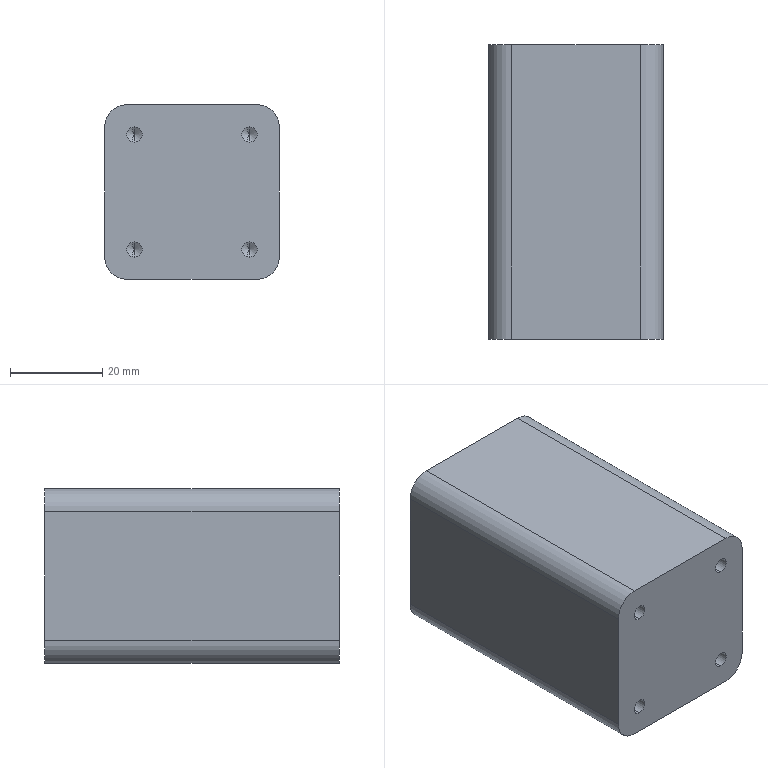Part | SolidWorks | features HoleWzd 2, ICE 2, Extrusion 1, Fillet 1 | 1 solid | 42 faces | box 38 x 64 x 38 mm | volume 90329 mm3 | cylinder 20 | cone 16 | plane 6 | commonest cylinder face diameters 3.3 x16 10 x4
STEP:
#1=CARTESIAN_POINT('',(-12.5,53.9,-14.15));
#2=VERTEX_POINT('',#1);
#3=CARTESIAN_POINT('',(-12.5,53.9,-10.85));
#4=VERTEX_POINT('',#3);
#5=CARTESIAN_POINT('',(-12.5,53.9,-12.5));
#6=DIRECTION('',(0.,1.,0.));
#7=DIRECTION('',(0.,0.,1.));
#8=AXIS2_PLACEMENT_3D('',#5,#6,#7);
#9=CIRCLE('',#8,1.65);
#10=EDGE_CURVE('',#2,#4,#9,.T.);
#11=ORIENTED_EDGE('',*,*,#10,.F.);
#12=CARTESIAN_POINT('',(-12.5,64.,-14.15));
#13=VERTEX_POINT('',#12);
#14=CARTESIAN_POINT('',(-12.5,64.,-14.15));
#15=DIRECTION('',(0.,1.,0.));
#16=VECTOR('',#15,1000.);
#17=LINE('',#14,#16);
#18=EDGE_CURVE('',#2,#13,#17,.T.);
#19=ORIENTED_EDGE('',*,*,#18,.T.);
#20=CARTESIAN_POINT('',(-12.5,64.,-10.85));
#21=VERTEX_POINT('',#20);
#22=CARTESIAN_POINT('',(-12.5,64.,-12.5));
#23=DIRECTION('',(0.,1.,0.));
#24=DIRECTION('',(0.,0.,1.));
#25=AXIS2_PLACEMENT_3D('',#22,#23,#24);
#26=CIRCLE('',#25,1.65);
#27=EDGE_CURVE('',#13,#21,#26,.T.);
#28=ORIENTED_EDGE('',*,*,#27,.T.);
#29=CARTESIAN_POINT('',(-12.5,64.,-10.85));
#30=DIRECTION('',(0.,1.,0.));
#31=VECTOR('',#30,1000.);
#32=LINE('',#29,#31);
#33=EDGE_CURVE('',#4,#21,#32,.T.);
#34=ORIENTED_EDGE('',*,*,#33,.F.);
#35=EDGE_LOOP('',(#11,#19,#28,#34));
#36=FACE_OUTER_BOUND('',#35,.T.);
#37=CARTESIAN_POINT('',(-12.5,64.,-12.5));
#38=DIRECTION('',(0.,1.,0.));
#39=DIRECTION('',(0.,0.,1.));
#40=AXIS2_PLACEMENT_3D('',#37,#38,#39);
#41=CYLINDRICAL_SURFACE('',#40,1.65);
#42=ADVANCED_FACE('',(#36),#41,.F.);
#43=CARTESIAN_POINT('',(-12.5,52.909,-12.5));
#44=VERTEX_POINT('',#43);
#45=CARTESIAN_POINT('',(-12.5,53.9,-10.85));
#46=DIRECTION('',(0.,0.515,0.8572));
#47=VECTOR('',#46,1000.);
#48=LINE('',#45,#47);
#49=EDGE_CURVE('',#44,#4,#48,.T.);
#50=ORIENTED_EDGE('',*,*,#49,.F.);
#51=CARTESIAN_POINT('',(-12.5,53.9,-14.15));
#52=DIRECTION('',(0.,0.515,-0.8572));
#53=VECTOR('',#52,1000.);
#54=LINE('',#51,#53);
#55=EDGE_CURVE('',#44,#2,#54,.T.);
#56=ORIENTED_EDGE('',*,*,#55,.T.);
#57=ORIENTED_EDGE('',*,*,#10,.T.);
#58=EDGE_LOOP('',(#50,#56,#57));
#59=FACE_OUTER_BOUND('',#58,.T.);
#60=CARTESIAN_POINT('',(-12.5,53.9,-12.5));
#61=DIRECTION('',(0.,1.,0.));
#62=DIRECTION('',(0.,0.,1.));
#63=AXIS2_PLACEMENT_3D('',#60,#61,#62);
#64=CONICAL_SURFACE('',#63,1.65,1.03);
#65=ADVANCED_FACE('',(#59),#64,.F.);
#66=CARTESIAN_POINT('',(12.5,53.9,-14.15));
#67=VERTEX_POINT('',#66);
#68=CARTESIAN_POINT('',(12.5,53.9,-10.85));
#69=VERTEX_POINT('',#68);
#70=CARTESIAN_POINT('',(12.5,53.9,-12.5));
#71=DIRECTION('',(0.,1.,0.));
#72=DIRECTION('',(0.,0.,1.));
#73=AXIS2_PLACEMENT_3D('',#70,#71,#72);
#74=CIRCLE('',#73,1.65);
#75=EDGE_CURVE('',#67,#69,#74,.T.);
#76=ORIENTED_EDGE('',*,*,#75,.F.);
#77=CARTESIAN_POINT('',(12.5,64.,-14.15));
#78=VERTEX_POINT('',#77);
#79=CARTESIAN_POINT('',(12.5,64.,-14.15));
#80=DIRECTION('',(0.,1.,0.));
#81=VECTOR('',#80,1000.);
#82=LINE('',#79,#81);
#83=EDGE_CURVE('',#67,#78,#82,.T.);
#84=ORIENTED_EDGE('',*,*,#83,.T.);
#85=CARTESIAN_POINT('',(12.5,64.,-10.85));
#86=VERTEX_POINT('',#85);
#87=CARTESIAN_POINT('',(12.5,64.,-12.5));
#88=DIRECTION('',(0.,1.,0.));
#89=DIRECTION('',(0.,0.,1.));
#90=AXIS2_PLACEMENT_3D('',#87,#88,#89);
#91=CIRCLE('',#90,1.65);
#92=EDGE_CURVE('',#78,#86,#91,.T.);
#93=ORIENTED_EDGE('',*,*,#92,.T.);
#94=CARTESIAN_POINT('',(12.5,64.,-10.85));
#95=DIRECTION('',(0.,1.,0.));
#96=VECTOR('',#95,1000.);
#97=LINE('',#94,#96);
#98=EDGE_CURVE('',#69,#86,#97,.T.);
#99=ORIENTED_EDGE('',*,*,#98,.F.);
#100=EDGE_LOOP('',(#76,#84,#93,#99));
#101=FACE_OUTER_BOUND('',#100,.T.);
#102=CARTESIAN_POINT('',(12.5,64.,-12.5));
#103=DIRECTION('',(0.,1.,0.));
#104=DIRECTION('',(0.,0.,1.));
#105=AXIS2_PLACEMENT_3D('',#102,#103,#104);
#106=CYLINDRICAL_SURFACE('',#105,1.65);
#107=ADVANCED_FACE('',(#101),#106,.F.);
#108=CARTESIAN_POINT('',(12.5,52.909,-12.5));
#109=VERTEX_POINT('',#108);
#110=CARTESIAN_POINT('',(12.5,53.9,-10.85));
#111=DIRECTION('',(0.,0.515,0.8572));
#112=VECTOR('',#111,1000.);
#113=LINE('',#110,#112);
#114=EDGE_CURVE('',#109,#69,#113,.T.);
#115=ORIENTED_EDGE('',*,*,#114,.F.);
#116=CARTESIAN_POINT('',(12.5,53.9,-14.15));
#117=DIRECTION('',(0.,0.515,-0.8572));
#118=VECTOR('',#117,1000.);
#119=LINE('',#116,#118);
#120=EDGE_CURVE('',#109,#67,#119,.T.);
#121=ORIENTED_EDGE('',*,*,#120,.T.);
#122=ORIENTED_EDGE('',*,*,#75,.T.);
#123=EDGE_LOOP('',(#115,#121,#122));
#124=FACE_OUTER_BOUND('',#123,.T.);
#125=CARTESIAN_POINT('',(12.5,53.9,-12.5));
#126=DIRECTION('',(0.,1.,0.));
#127=DIRECTION('',(0.,0.,1.));
#128=AXIS2_PLACEMENT_3D('',#125,#126,#127);
#129=CONICAL_SURFACE('',#128,1.65,1.03);
#130=ADVANCED_FACE('',(#124),#129,.F.);
#131=CARTESIAN_POINT('',(12.5,53.9,10.85));
#132=VERTEX_POINT('',#131);
#133=CARTESIAN_POINT('',(12.5,53.9,14.15));
#134=VERTEX_POINT('',#133);
#135=CARTESIAN_POINT('',(12.5,53.9,12.5));
#136=DIRECTION('',(0.,1.,0.));
#137=DIRECTION('',(0.,0.,1.));
#138=AXIS2_PLACEMENT_3D('',#135,#136,#137);
#139=CIRCLE('',#138,1.65);
#140=EDGE_CURVE('',#132,#134,#139,.T.);
#141=ORIENTED_EDGE('',*,*,#140,.F.);
#142=CARTESIAN_POINT('',(12.5,64.,10.85));
#143=VERTEX_POINT('',#142);
#144=CARTESIAN_POINT('',(12.5,64.,10.85));
#145=DIRECTION('',(0.,1.,0.));
#146=VECTOR('',#145,1000.);
#147=LINE('',#144,#146);
#148=EDGE_CURVE('',#132,#143,#147,.T.);
#149=ORIENTED_EDGE('',*,*,#148,.T.);
#150=CARTESIAN_POINT('',(12.5,64.,14.15));
#151=VERTEX_POINT('',#150);
#152=CARTESIAN_POINT('',(12.5,64.,12.5));
#153=DIRECTION('',(0.,1.,0.));
#154=DIRECTION('',(0.,0.,1.));
#155=AXIS2_PLACEMENT_3D('',#152,#153,#154);
#156=CIRCLE('',#155,1.65);
#157=EDGE_CURVE('',#143,#151,#156,.T.);
#158=ORIENTED_EDGE('',*,*,#157,.T.);
#159=CARTESIAN_POINT('',(12.5,64.,14.15));
#160=DIRECTION('',(0.,1.,0.));
#161=VECTOR('',#160,1000.);
#162=LINE('',#159,#161);
#163=EDGE_CURVE('',#134,#151,#162,.T.);
#164=ORIENTED_EDGE('',*,*,#163,.F.);
#165=EDGE_LOOP('',(#141,#149,#158,#164));
#166=FACE_OUTER_BOUND('',#165,.T.);
#167=CARTESIAN_POINT('',(12.5,64.,12.5));
#168=DIRECTION('',(0.,1.,0.));
#169=DIRECTION('',(0.,0.,1.));
#170=AXIS2_PLACEMENT_3D('',#167,#168,#169);
#171=CYLINDRICAL_SURFACE('',#170,1.65);
#172=ADVANCED_FACE('',(#166),#171,.F.);
#173=CARTESIAN_POINT('',(12.5,52.909,12.5));
#174=VERTEX_POINT('',#173);
#175=CARTESIAN_POINT('',(12.5,53.9,14.15));
#176=DIRECTION('',(0.,0.515,0.8572));
#177=VECTOR('',#176,1000.);
#178=LINE('',#175,#177);
#179=EDGE_CURVE('',#174,#134,#178,.T.);
#180=ORIENTED_EDGE('',*,*,#179,.F.);
#181=CARTESIAN_POINT('',(12.5,53.9,10.85));
#182=DIRECTION('',(0.,0.515,-0.8572));
#183=VECTOR('',#182,1000.);
#184=LINE('',#181,#183);
#185=EDGE_CURVE('',#174,#132,#184,.T.);
#186=ORIENTED_EDGE('',*,*,#185,.T.);
#187=ORIENTED_EDGE('',*,*,#140,.T.);
#188=EDGE_LOOP('',(#180,#186,#187));
#189=FACE_OUTER_BOUND('',#188,.T.);
#190=CARTESIAN_POINT('',(12.5,53.9,12.5));
#191=DIRECTION('',(0.,1.,0.));
#192=DIRECTION('',(0.,0.,1.));
#193=AXIS2_PLACEMENT_3D('',#190,#191,#192);
#194=CONICAL_SURFACE('',#193,1.65,1.03);
#195=ADVANCED_FACE('',(#189),#194,.F.);
#196=CARTESIAN_POINT('',(-12.5,53.9,10.85));
#197=VERTEX_POINT('',#196);
#198=CARTESIAN_POINT('',(-12.5,53.9,14.15));
#199=VERTEX_POINT('',#198);
#200=CARTESIAN_POINT('',(-12.5,53.9,12.5));
#201=DIRECTION('',(0.,1.,0.));
#202=DIRECTION('',(0.,0.,1.));
#203=AXIS2_PLACEMENT_3D('',#200,#201,#202);
#204=CIRCLE('',#203,1.65);
#205=EDGE_CURVE('',#197,#199,#204,.T.);
#206=ORIENTED_EDGE('',*,*,#205,.F.);
#207=CARTESIAN_POINT('',(-12.5,64.,10.85));
#208=VERTEX_POINT('',#207);
#209=CARTESIAN_POINT('',(-12.5,64.,10.85));
#210=DIRECTION('',(0.,1.,0.));
#211=VECTOR('',#210,1000.);
#212=LINE('',#209,#211);
#213=EDGE_CURVE('',#197,#208,#212,.T.);
#214=ORIENTED_EDGE('',*,*,#213,.T.);
#215=CARTESIAN_POINT('',(-12.5,64.,14.15));
#216=VERTEX_POINT('',#215);
#217=CARTESIAN_POINT('',(-12.5,64.,12.5));
#218=DIRECTION('',(0.,1.,0.));
#219=DIRECTION('',(0.,0.,1.));
#220=AXIS2_PLACEMENT_3D('',#217,#218,#219);
#221=CIRCLE('',#220,1.65);
#222=EDGE_CURVE('',#208,#216,#221,.T.);
#223=ORIENTED_EDGE('',*,*,#222,.T.);
#224=CARTESIAN_POINT('',(-12.5,64.,14.15));
#225=DIRECTION('',(0.,1.,0.));
#226=VECTOR('',#225,1000.);
#227=LINE('',#224,#226);
#228=EDGE_CURVE('',#199,#216,#227,.T.);
#229=ORIENTED_EDGE('',*,*,#228,.F.);
#230=EDGE_LOOP('',(#206,#214,#223,#229));
#231=FACE_OUTER_BOUND('',#230,.T.);
#232=CARTESIAN_POINT('',(-12.5,64.,12.5));
#233=DIRECTION('',(0.,1.,0.));
#234=DIRECTION('',(0.,0.,1.));
#235=AXIS2_PLACEMENT_3D('',#232,#233,#234);
#236=CYLINDRICAL_SURFACE('',#235,1.65);
#237=ADVANCED_FACE('',(#231),#236,.F.);
#238=CARTESIAN_POINT('',(-12.5,52.909,12.5));
#239=VERTEX_POINT('',#238);
#240=CARTESIAN_POINT('',(-12.5,53.9,14.15));
#241=DIRECTION('',(0.,0.515,0.8572));
#242=VECTOR('',#241,1000.);
#243=LINE('',#240,#242);
#244=EDGE_CURVE('',#239,#199,#243,.T.);
#245=ORIENTED_EDGE('',*,*,#244,.F.);
#246=CARTESIAN_POINT('',(-12.5,53.9,10.85));
#247=DIRECTION('',(0.,0.515,-0.8572));
#248=VECTOR('',#247,1000.);
#249=LINE('',#246,#248);
#250=EDGE_CURVE('',#239,#197,#249,.T.);
#251=ORIENTED_EDGE('',*,*,#250,.T.);
#252=ORIENTED_EDGE('',*,*,#205,.T.);
#253=EDGE_LOOP('',(#245,#251,#252));
#254=FACE_OUTER_BOUND('',#253,.T.);
#255=CARTESIAN_POINT('',(-12.5,53.9,12.5));
#256=DIRECTION('',(0.,1.,0.));
#257=DIRECTION('',(0.,0.,1.));
#258=AXIS2_PLACEMENT_3D('',#255,#256,#257);
#259=CONICAL_SURFACE('',#258,1.65,1.03);
#260=ADVANCED_FACE('',(#254),#259,.F.);
#261=CARTESIAN_POINT('',(-12.5,10.1,-10.85));
#262=VERTEX_POINT('',#261);
#263=CARTESIAN_POINT('',(-12.5,10.1,-14.15));
#264=VERTEX_POINT('',#263);
#265=CARTESIAN_POINT('',(-12.5,10.1,-12.5));
#266=DIRECTION('',(0.,-1.,0.));
#267=DIRECTION('',(0.,0.,-1.));
#268=AXIS2_PLACEMENT_3D('',#265,#266,#267);
#269=CIRCLE('',#268,1.65);
#270=EDGE_CURVE('',#262,#264,#269,.T.);
#271=ORIENTED_EDGE('',*,*,#270,.F.);
#272=CARTESIAN_POINT('',(-12.5,0.,-10.85));
#273=VERTEX_POINT('',#272);
#274=CARTESIAN_POINT('',(-12.5,0.,-10.85));
#275=DIRECTION('',(0.,-1.,0.));
#276=VECTOR('',#275,1000.);
#277=LINE('',#274,#276);
#278=EDGE_CURVE('',#262,#273,#277,.T.);
#279=ORIENTED_EDGE('',*,*,#278,.T.);
#280=CARTESIAN_POINT('',(-12.5,0.,-14.15));
#281=VERTEX_POINT('',#280);
#282=CARTESIAN_POINT('',(-12.5,0.,-12.5));
#283=DIRECTION('',(0.,-1.,0.));
#284=DIRECTION('',(0.,0.,-1.));
#285=AXIS2_PLACEMENT_3D('',#282,#283,#284);
#286=CIRCLE('',#285,1.65);
#287=EDGE_CURVE('',#273,#281,#286,.T.);
#288=ORIENTED_EDGE('',*,*,#287,.T.);
#289=CARTESIAN_POINT('',(-12.5,0.,-14.15));
#290=DIRECTION('',(0.,-1.,0.));
#291=VECTOR('',#290,1000.);
#292=LINE('',#289,#291);
#293=EDGE_CURVE('',#264,#281,#292,.T.);
#294=ORIENTED_EDGE('',*,*,#293,.F.);
#295=EDGE_LOOP('',(#271,#279,#288,#294));
#296=FACE_OUTER_BOUND('',#295,.T.);
#297=CARTESIAN_POINT('',(-12.5,0.,-12.5));
#298=DIRECTION('',(0.,-1.,0.));
#299=DIRECTION('',(0.,0.,-1.));
#300=AXIS2_PLACEMENT_3D('',#297,#298,#299);
#301=CYLINDRICAL_SURFACE('',#300,1.65);
#302=ADVANCED_FACE('',(#296),#301,.F.);
#303=CARTESIAN_POINT('',(-12.5,11.091,-12.5));
#304=VERTEX_POINT('',#303);
#305=CARTESIAN_POINT('',(-12.5,10.1,-14.15));
#306=DIRECTION('',(0.,-0.515,-0.8572));
#307=VECTOR('',#306,1000.);
#308=LINE('',#305,#307);
#309=EDGE_CURVE('',#304,#264,#308,.T.);
#310=ORIENTED_EDGE('',*,*,#309,.F.);
#311=CARTESIAN_POINT('',(-12.5,10.1,-10.85));
#312=DIRECTION('',(0.,-0.515,0.8572));
#313=VECTOR('',#312,1000.);
#314=LINE('',#311,#313);
#315=EDGE_CURVE('',#304,#262,#314,.T.);
#316=ORIENTED_EDGE('',*,*,#315,.T.);
#317=ORIENTED_EDGE('',*,*,#270,.T.);
#318=EDGE_LOOP('',(#310,#316,#317));
#319=FACE_OUTER_BOUND('',#318,.T.);
#320=CARTESIAN_POINT('',(-12.5,10.1,-12.5));
#321=DIRECTION('',(0.,-1.,0.));
#322=DIRECTION('',(0.,0.,-1.));
#323=AXIS2_PLACEMENT_3D('',#320,#321,#322);
#324=CONICAL_SURFACE('',#323,1.65,1.03);
#325=ADVANCED_FACE('',(#319),#324,.F.);
#326=CARTESIAN_POINT('',(12.5,10.1,-10.85));
#327=VERTEX_POINT('',#326);
#328=CARTESIAN_POINT('',(12.5,10.1,-14.15));
#329=VERTEX_POINT('',#328);
#330=CARTESIAN_POINT('',(12.5,10.1,-12.5));
#331=DIRECTION('',(0.,-1.,0.));
#332=DIRECTION('',(0.,0.,-1.));
#333=AXIS2_PLACEMENT_3D('',#330,#331,#332);
#334=CIRCLE('',#333,1.65);
#335=EDGE_CURVE('',#327,#329,#334,.T.);
#336=ORIENTED_EDGE('',*,*,#335,.F.);
#337=CARTESIAN_POINT('',(12.5,0.,-10.85));
#338=VERTEX_POINT('',#337);
#339=CARTESIAN_POINT('',(12.5,0.,-10.85));
#340=DIRECTION('',(0.,-1.,0.));
#341=VECTOR('',#340,1000.);
#342=LINE('',#339,#341);
#343=EDGE_CURVE('',#327,#338,#342,.T.);
#344=ORIENTED_EDGE('',*,*,#343,.T.);
#345=CARTESIAN_POINT('',(12.5,0.,-14.15));
#346=VERTEX_POINT('',#345);
#347=CARTESIAN_POINT('',(12.5,0.,-12.5));
#348=DIRECTION('',(0.,-1.,0.));
#349=DIRECTION('',(0.,0.,-1.));
#350=AXIS2_PLACEMENT_3D('',#347,#348,#349);
#351=CIRCLE('',#350,1.65);
#352=EDGE_CURVE('',#338,#346,#351,.T.);
#353=ORIENTED_EDGE('',*,*,#352,.T.);
#354=CARTESIAN_POINT('',(12.5,0.,-14.15));
#355=DIRECTION('',(0.,-1.,0.));
#356=VECTOR('',#355,1000.);
#357=LINE('',#354,#356);
#358=EDGE_CURVE('',#329,#346,#357,.T.);
#359=ORIENTED_EDGE('',*,*,#358,.F.);
#360=EDGE_LOOP('',(#336,#344,#353,#359));
#361=FACE_OUTER_BOUND('',#360,.T.);
#362=CARTESIAN_POINT('',(12.5,0.,-12.5));
#363=DIRECTION('',(0.,-1.,0.));
#364=DIRECTION('',(0.,0.,-1.));
#365=AXIS2_PLACEMENT_3D('',#362,#363,#364);
#366=CYLINDRICAL_SURFACE('',#365,1.65);
#367=ADVANCED_FACE('',(#361),#366,.F.);
#368=CARTESIAN_POINT('',(12.5,11.091,-12.5));
#369=VERTEX_POINT('',#368);
#370=CARTESIAN_POINT('',(12.5,10.1,-14.15));
#371=DIRECTION('',(0.,-0.515,-0.8572));
#372=VECTOR('',#371,1000.);
#373=LINE('',#370,#372);
#374=EDGE_CURVE('',#369,#329,#373,.T.);
#375=ORIENTED_EDGE('',*,*,#374,.F.);
#376=CARTESIAN_POINT('',(12.5,10.1,-10.85));
#377=DIRECTION('',(0.,-0.515,0.8572));
#378=VECTOR('',#377,1000.);
#379=LINE('',#376,#378);
#380=EDGE_CURVE('',#369,#327,#379,.T.);
#381=ORIENTED_EDGE('',*,*,#380,.T.);
#382=ORIENTED_EDGE('',*,*,#335,.T.);
#383=EDGE_LOOP('',(#375,#381,#382));
#384=FACE_OUTER_BOUND('',#383,.T.);
#385=CARTESIAN_POINT('',(12.5,10.1,-12.5));
#386=DIRECTION('',(0.,-1.,0.));
#387=DIRECTION('',(0.,0.,-1.));
#388=AXIS2_PLACEMENT_3D('',#385,#386,#387);
#389=CONICAL_SURFACE('',#388,1.65,1.03);
#390=ADVANCED_FACE('',(#384),#389,.F.);
#391=CARTESIAN_POINT('',(-12.5,10.1,14.15));
#392=VERTEX_POINT('',#391);
#393=CARTESIAN_POINT('',(-12.5,10.1,10.85));
#394=VERTEX_POINT('',#393);
#395=CARTESIAN_POINT('',(-12.5,10.1,12.5));
#396=DIRECTION('',(0.,-1.,0.));
#397=DIRECTION('',(0.,0.,-1.));
#398=AXIS2_PLACEMENT_3D('',#395,#396,#397);
#399=CIRCLE('',#398,1.65);
#400=EDGE_CURVE('',#392,#394,#399,.T.);
#401=ORIENTED_EDGE('',*,*,#400,.F.);
#402=CARTESIAN_POINT('',(-12.5,0.,14.15));
#403=VERTEX_POINT('',#402);
#404=CARTESIAN_POINT('',(-12.5,0.,14.15));
#405=DIRECTION('',(0.,-1.,0.));
#406=VECTOR('',#405,1000.);
#407=LINE('',#404,#406);
#408=EDGE_CURVE('',#392,#403,#407,.T.);
#409=ORIENTED_EDGE('',*,*,#408,.T.);
#410=CARTESIAN_POINT('',(-12.5,0.,10.85));
#411=VERTEX_POINT('',#410);
#412=CARTESIAN_POINT('',(-12.5,0.,12.5));
#413=DIRECTION('',(0.,-1.,0.));
#414=DIRECTION('',(0.,0.,-1.));
#415=AXIS2_PLACEMENT_3D('',#412,#413,#414);
#416=CIRCLE('',#415,1.65);
#417=EDGE_CURVE('',#403,#411,#416,.T.);
#418=ORIENTED_EDGE('',*,*,#417,.T.);
#419=CARTESIAN_POINT('',(-12.5,0.,10.85));
#420=DIRECTION('',(0.,-1.,0.));
#421=VECTOR('',#420,1000.);
#422=LINE('',#419,#421);
#423=EDGE_CURVE('',#394,#411,#422,.T.);
#424=ORIENTED_EDGE('',*,*,#423,.F.);
#425=EDGE_LOOP('',(#401,#409,#418,#424));
#426=FACE_OUTER_BOUND('',#425,.T.);
#427=CARTESIAN_POINT('',(-12.5,0.,12.5));
#428=DIRECTION('',(0.,-1.,0.));
#429=DIRECTION('',(0.,0.,-1.));
#430=AXIS2_PLACEMENT_3D('',#427,#428,#429);
#431=CYLINDRICAL_SURFACE('',#430,1.65);
#432=ADVANCED_FACE('',(#426),#431,.F.);
#433=CARTESIAN_POINT('',(-12.5,11.091,12.5));
#434=VERTEX_POINT('',#433);
#435=CARTESIAN_POINT('',(-12.5,10.1,10.85));
#436=DIRECTION('',(0.,-0.515,-0.8572));
#437=VECTOR('',#436,1000.);
#438=LINE('',#435,#437);
#439=EDGE_CURVE('',#434,#394,#438,.T.);
#440=ORIENTED_EDGE('',*,*,#439,.F.);
#441=CARTESIAN_POINT('',(-12.5,10.1,14.15));
#442=DIRECTION('',(0.,-0.515,0.8572));
#443=VECTOR('',#442,1000.);
#444=LINE('',#441,#443);
#445=EDGE_CURVE('',#434,#392,#444,.T.);
#446=ORIENTED_EDGE('',*,*,#445,.T.);
#447=ORIENTED_EDGE('',*,*,#400,.T.);
#448=EDGE_LOOP('',(#440,#446,#447));
#449=FACE_OUTER_BOUND('',#448,.T.);
#450=CARTESIAN_POINT('',(-12.5,10.1,12.5));
#451=DIRECTION('',(0.,-1.,0.));
#452=DIRECTION('',(0.,0.,-1.));
#453=AXIS2_PLACEMENT_3D('',#450,#451,#452);
#454=CONICAL_SURFACE('',#453,1.65,1.03);
#455=ADVANCED_FACE('',(#449),#454,.F.);
#456=CARTESIAN_POINT('',(12.5,10.1,14.15));
#457=VERTEX_POINT('',#456);
#458=CARTESIAN_POINT('',(12.5,10.1,10.85));
#459=VERTEX_POINT('',#458);
#460=CARTESIAN_POINT('',(12.5,10.1,12.5));
#461=DIRECTION('',(0.,-1.,0.));
#462=DIRECTION('',(0.,0.,-1.));
#463=AXIS2_PLACEMENT_3D('',#460,#461,#462);
#464=CIRCLE('',#463,1.65);
#465=EDGE_CURVE('',#457,#459,#464,.T.);
#466=ORIENTED_EDGE('',*,*,#465,.F.);
#467=CARTESIAN_POINT('',(12.5,0.,14.15));
#468=VERTEX_POINT('',#467);
#469=CARTESIAN_POINT('',(12.5,0.,14.15));
#470=DIRECTION('',(0.,-1.,0.));
#471=VECTOR('',#470,1000.);
#472=LINE('',#469,#471);
#473=EDGE_CURVE('',#457,#468,#472,.T.);
#474=ORIENTED_EDGE('',*,*,#473,.T.);
#475=CARTESIAN_POINT('',(12.5,0.,10.85));
#476=VERTEX_POINT('',#475);
#477=CARTESIAN_POINT('',(12.5,0.,12.5));
#478=DIRECTION('',(0.,-1.,0.));
#479=DIRECTION('',(0.,0.,-1.));
#480=AXIS2_PLACEMENT_3D('',#477,#478,#479);
#481=CIRCLE('',#480,1.65);
#482=EDGE_CURVE('',#468,#476,#481,.T.);
#483=ORIENTED_EDGE('',*,*,#482,.T.);
#484=CARTESIAN_POINT('',(12.5,0.,10.85));
#485=DIRECTION('',(0.,-1.,0.));
#486=VECTOR('',#485,1000.);
#487=LINE('',#484,#486);
#488=EDGE_CURVE('',#459,#476,#487,.T.);
#489=ORIENTED_EDGE('',*,*,#488,.F.);
#490=EDGE_LOOP('',(#466,#474,#483,#489));
#491=FACE_OUTER_BOUND('',#490,.T.);
#492=CARTESIAN_POINT('',(12.5,0.,12.5));
#493=DIRECTION('',(0.,-1.,0.));
#494=DIRECTION('',(0.,0.,-1.));
#495=AXIS2_PLACEMENT_3D('',#492,#493,#494);
#496=CYLINDRICAL_SURFACE('',#495,1.65);
#497=ADVANCED_FACE('',(#491),#496,.F.);
#498=CARTESIAN_POINT('',(12.5,11.091,12.5));
#499=VERTEX_POINT('',#498);
#500=CARTESIAN_POINT('',(12.5,10.1,10.85));
#501=DIRECTION('',(0.,-0.515,-0.8572));
#502=VECTOR('',#501,1000.);
#503=LINE('',#500,#502);
#504=EDGE_CURVE('',#499,#459,#503,.T.);
#505=ORIENTED_EDGE('',*,*,#504,.F.);
#506=CARTESIAN_POINT('',(12.5,10.1,14.15));
#507=DIRECTION('',(0.,-0.515,0.8572));
#508=VECTOR('',#507,1000.);
#509=LINE('',#506,#508);
#510=EDGE_CURVE('',#499,#457,#509,.T.);
#511=ORIENTED_EDGE('',*,*,#510,.T.);
#512=ORIENTED_EDGE('',*,*,#465,.T.);
#513=EDGE_LOOP('',(#505,#511,#512));
#514=FACE_OUTER_BOUND('',#513,.T.);
#515=CARTESIAN_POINT('',(12.5,10.1,12.5));
#516=DIRECTION('',(0.,-1.,0.));
#517=DIRECTION('',(0.,0.,-1.));
#518=AXIS2_PLACEMENT_3D('',#515,#516,#517);
#519=CONICAL_SURFACE('',#518,1.65,1.03);
#520=ADVANCED_FACE('',(#514),#519,.F.);
#521=CARTESIAN_POINT('',(19.,0.,14.));
#522=VERTEX_POINT('',#521);
#523=CARTESIAN_POINT('',(19.,0.,-14.));
#524=VERTEX_POINT('',#523);
#525=CARTESIAN_POINT('',(19.,0.,-34.));
#526=DIRECTION('',(0.,0.,-1.));
#527=VECTOR('',#526,1000.);
#528=LINE('',#525,#527);
#529=EDGE_CURVE('',#522,#524,#528,.T.);
#530=ORIENTED_EDGE('',*,*,#529,.T.);
#531=CARTESIAN_POINT('',(19.,64.,-14.));
#532=VERTEX_POINT('',#531);
#533=CARTESIAN_POINT('',(19.,10.,-14.));
#534=DIRECTION('',(0.,1.,0.));
#535=VECTOR('',#534,1000.);
#536=LINE('',#533,#535);
#537=EDGE_CURVE('',#524,#532,#536,.T.);
#538=ORIENTED_EDGE('',*,*,#537,.T.);
#539=CARTESIAN_POINT('',(19.,64.,14.));
#540=VERTEX_POINT('',#539);
#541=CARTESIAN_POINT('',(19.,64.,-19.));
#542=DIRECTION('',(0.,0.,-1.));
#543=VECTOR('',#542,1000.);
#544=LINE('',#541,#543);
#545=EDGE_CURVE('',#540,#532,#544,.T.);
#546=ORIENTED_EDGE('',*,*,#545,.F.);
#547=CARTESIAN_POINT('',(19.,10.,14.));
#548=DIRECTION('',(0.,-1.,0.));
#549=VECTOR('',#548,1000.);
#550=LINE('',#547,#549);
#551=EDGE_CURVE('',#540,#522,#550,.T.);
#552=ORIENTED_EDGE('',*,*,#551,.T.);
#553=EDGE_LOOP('',(#530,#538,#546,#552));
#554=FACE_OUTER_BOUND('',#553,.T.);
#555=CARTESIAN_POINT('',(19.,10.,-34.));
#556=DIRECTION('',(-1.,0.,0.));
#557=DIRECTION('',(0.,0.,1.));
#558=AXIS2_PLACEMENT_3D('',#555,#556,#557);
#559=PLANE('',#558);
#560=ADVANCED_FACE('',(#554),#559,.F.);
#561=CARTESIAN_POINT('',(-19.,0.,-14.));
#562=VERTEX_POINT('',#561);
#563=CARTESIAN_POINT('',(-19.,0.,14.));
#564=VERTEX_POINT('',#563);
#565=CARTESIAN_POINT('',(-19.,0.,-34.));
#566=DIRECTION('',(0.,0.,1.));
#567=VECTOR('',#566,1000.);
#568=LINE('',#565,#567);
#569=EDGE_CURVE('',#562,#564,#568,.T.);
#570=ORIENTED_EDGE('',*,*,#569,.T.);
#571=CARTESIAN_POINT('',(-19.,64.,14.));
#572=VERTEX_POINT('',#571);
#573=CARTESIAN_POINT('',(-19.,10.,14.));
#574=DIRECTION('',(0.,1.,0.));
#575=VECTOR('',#574,1000.);
#576=LINE('',#573,#575);
#577=EDGE_CURVE('',#564,#572,#576,.T.);
#578=ORIENTED_EDGE('',*,*,#577,.T.);
#579=CARTESIAN_POINT('',(-19.,64.,-14.));
#580=VERTEX_POINT('',#579);
#581=CARTESIAN_POINT('',(-19.,64.,-19.));
#582=DIRECTION('',(0.,0.,1.));
#583=VECTOR('',#582,1000.);
#584=LINE('',#581,#583);
#585=EDGE_CURVE('',#580,#572,#584,.T.);
#586=ORIENTED_EDGE('',*,*,#585,.F.);
#587=CARTESIAN_POINT('',(-19.,10.,-14.));
#588=DIRECTION('',(0.,-1.,0.));
#589=VECTOR('',#588,1000.);
#590=LINE('',#587,#589);
#591=EDGE_CURVE('',#580,#562,#590,.T.);
#592=ORIENTED_EDGE('',*,*,#591,.T.);
#593=EDGE_LOOP('',(#570,#578,#586,#592));
#594=FACE_OUTER_BOUND('',#593,.T.);
#595=CARTESIAN_POINT('',(-19.,10.,-34.));
#596=DIRECTION('',(1.,0.,0.));
#597=DIRECTION('',(0.,0.,-1.));
#598=AXIS2_PLACEMENT_3D('',#595,#596,#597);
#599=PLANE('',#598);
#600=ADVANCED_FACE('',(#594),#599,.F.);
#601=CARTESIAN_POINT('',(-12.5,0.,-12.5));
#602=DIRECTION('',(0.,-1.,0.));
#603=DIRECTION('',(0.,0.,-1.));
#604=AXIS2_PLACEMENT_3D('',#601,#602,#603);
#605=CIRCLE('',#604,1.65);
#606=EDGE_CURVE('',#281,#273,#605,.T.);
#607=ORIENTED_EDGE('',*,*,#606,.F.);
#608=ORIENTED_EDGE('',*,*,#287,.F.);
#609=EDGE_LOOP('',(#607,#608));
#610=FACE_BOUND('',#609,.T.);
#611=CARTESIAN_POINT('',(12.5,0.,-12.5));
#612=DIRECTION('',(0.,-1.,0.));
#613=DIRECTION('',(0.,0.,-1.));
#614=AXIS2_PLACEMENT_3D('',#611,#612,#613);
#615=CIRCLE('',#614,1.65);
#616=EDGE_CURVE('',#346,#338,#615,.T.);
#617=ORIENTED_EDGE('',*,*,#616,.F.);
#618=ORIENTED_EDGE('',*,*,#352,.F.);
#619=EDGE_LOOP('',(#617,#618));
#620=FACE_BOUND('',#619,.T.);
#621=CARTESIAN_POINT('',(-12.5,0.,12.5));
#622=DIRECTION('',(0.,-1.,0.));
#623=DIRECTION('',(0.,0.,-1.));
#624=AXIS2_PLACEMENT_3D('',#621,#622,#623);
#625=CIRCLE('',#624,1.65);
#626=EDGE_CURVE('',#411,#403,#625,.T.);
#627=ORIENTED_EDGE('',*,*,#626,.F.);
#628=ORIENTED_EDGE('',*,*,#417,.F.);
#629=EDGE_LOOP('',(#627,#628));
#630=FACE_BOUND('',#629,.T.);
#631=CARTESIAN_POINT('',(12.5,0.,12.5));
#632=DIRECTION('',(0.,-1.,0.));
#633=DIRECTION('',(0.,0.,-1.));
#634=AXIS2_PLACEMENT_3D('',#631,#632,#633);
#635=CIRCLE('',#634,1.65);
#636=EDGE_CURVE('',#476,#468,#635,.T.);
#637=ORIENTED_EDGE('',*,*,#636,.F.);
#638=ORIENTED_EDGE('',*,*,#482,.F.);
#639=EDGE_LOOP('',(#637,#638));
#640=FACE_BOUND('',#639,.T.);
#641=CARTESIAN_POINT('',(14.,0.,19.));
#642=VERTEX_POINT('',#641);
#643=CARTESIAN_POINT('',(14.,0.,14.));
#644=DIRECTION('',(0.,1.,0.));
#645=DIRECTION('',(0.,0.,1.));
#646=AXIS2_PLACEMENT_3D('',#643,#644,#645);
#647=CIRCLE('',#646,5.);
#648=EDGE_CURVE('',#642,#522,#647,.T.);
#649=ORIENTED_EDGE('',*,*,#648,.F.);
#650=CARTESIAN_POINT('',(-14.,0.,19.));
#651=VERTEX_POINT('',#650);
#652=CARTESIAN_POINT('',(-14.,0.,19.));
#653=DIRECTION('',(1.,0.,0.));
#654=VECTOR('',#653,1000.);
#655=LINE('',#652,#654);
#656=EDGE_CURVE('',#651,#642,#655,.T.);
#657=ORIENTED_EDGE('',*,*,#656,.F.);
#658=CARTESIAN_POINT('',(-14.,0.,14.));
#659=DIRECTION('',(0.,1.,0.));
#660=DIRECTION('',(0.,0.,1.));
#661=AXIS2_PLACEMENT_3D('',#658,#659,#660);
#662=CIRCLE('',#661,5.);
#663=EDGE_CURVE('',#564,#651,#662,.T.);
#664=ORIENTED_EDGE('',*,*,#663,.F.);
#665=ORIENTED_EDGE('',*,*,#569,.F.);
#666=CARTESIAN_POINT('',(-14.,0.,-19.));
#667=VERTEX_POINT('',#666);
#668=CARTESIAN_POINT('',(-14.,0.,-14.));
#669=DIRECTION('',(0.,1.,0.));
#670=DIRECTION('',(0.,0.,1.));
#671=AXIS2_PLACEMENT_3D('',#668,#669,#670);
#672=CIRCLE('',#671,5.);
#673=EDGE_CURVE('',#667,#562,#672,.T.);
#674=ORIENTED_EDGE('',*,*,#673,.F.);
#675=CARTESIAN_POINT('',(14.,0.,-19.));
#676=VERTEX_POINT('',#675);
#677=CARTESIAN_POINT('',(-14.,0.,-19.));
#678=DIRECTION('',(-1.,0.,0.));
#679=VECTOR('',#678,1000.);
#680=LINE('',#677,#679);
#681=EDGE_CURVE('',#676,#667,#680,.T.);
#682=ORIENTED_EDGE('',*,*,#681,.F.);
#683=CARTESIAN_POINT('',(14.,0.,-14.));
#684=DIRECTION('',(0.,1.,0.));
#685=DIRECTION('',(0.,0.,-1.));
#686=AXIS2_PLACEMENT_3D('',#683,#684,#685);
#687=CIRCLE('',#686,5.);
#688=EDGE_CURVE('',#524,#676,#687,.T.);
#689=ORIENTED_EDGE('',*,*,#688,.F.);
#690=ORIENTED_EDGE('',*,*,#529,.F.);
#691=EDGE_LOOP('',(#649,#657,#664,#665,#674,#682,#689,#690));
#692=FACE_OUTER_BOUND('',#691,.T.);
#693=CARTESIAN_POINT('',(0.,0.,0.));
#694=DIRECTION('',(0.,1.,0.));
#695=DIRECTION('',(0.,0.,1.));
#696=AXIS2_PLACEMENT_3D('',#693,#694,#695);
#697=PLANE('',#696);
#698=ADVANCED_FACE('',(#610,#620,#630,#640,#692),#697,.F.);
#699=CARTESIAN_POINT('',(14.,64.,-19.));
#700=VERTEX_POINT('',#699);
#701=CARTESIAN_POINT('',(-14.,64.,-19.));
#702=VERTEX_POINT('',#701);
#703=CARTESIAN_POINT('',(-19.,64.,-19.));
#704=DIRECTION('',(-1.,0.,0.));
#705=VECTOR('',#704,1000.);
#706=LINE('',#703,#705);
#707=EDGE_CURVE('',#700,#702,#706,.T.);
#708=ORIENTED_EDGE('',*,*,#707,.F.);
#709=CARTESIAN_POINT('',(14.,64.,-19.));
#710=DIRECTION('',(0.,-1.,0.));
#711=VECTOR('',#710,1000.);
#712=LINE('',#709,#711);
#713=EDGE_CURVE('',#700,#676,#712,.T.);
#714=ORIENTED_EDGE('',*,*,#713,.T.);
#715=ORIENTED_EDGE('',*,*,#681,.T.);
#716=CARTESIAN_POINT('',(-14.,64.,-19.));
#717=DIRECTION('',(0.,1.,0.));
#718=VECTOR('',#717,1000.);
#719=LINE('',#716,#718);
#720=EDGE_CURVE('',#667,#702,#719,.T.);
#721=ORIENTED_EDGE('',*,*,#720,.T.);
#722=EDGE_LOOP('',(#708,#714,#715,#721));
#723=FACE_OUTER_BOUND('',#722,.T.);
#724=CARTESIAN_POINT('',(-19.,64.,-19.));
#725=DIRECTION('',(0.,0.,1.));
#726=DIRECTION('',(1.,0.,0.));
#727=AXIS2_PLACEMENT_3D('',#724,#725,#726);
#728=PLANE('',#727);
#729=ADVANCED_FACE('',(#723),#728,.F.);
#730=CARTESIAN_POINT('',(-14.,64.,19.));
#731=VERTEX_POINT('',#730);
#732=CARTESIAN_POINT('',(-14.,64.,19.));
#733=DIRECTION('',(0.,-1.,0.));
#734=VECTOR('',#733,1000.);
#735=LINE('',#732,#734);
#736=EDGE_CURVE('',#731,#651,#735,.T.);
#737=ORIENTED_EDGE('',*,*,#736,.T.);
#738=ORIENTED_EDGE('',*,*,#656,.T.);
#739=CARTESIAN_POINT('',(14.,64.,19.));
#740=VERTEX_POINT('',#739);
#741=CARTESIAN_POINT('',(14.,64.,19.));
#742=DIRECTION('',(0.,1.,0.));
#743=VECTOR('',#742,1000.);
#744=LINE('',#741,#743);
#745=EDGE_CURVE('',#642,#740,#744,.T.);
#746=ORIENTED_EDGE('',*,*,#745,.T.);
#747=CARTESIAN_POINT('',(-19.,64.,19.));
#748=DIRECTION('',(1.,0.,0.));
#749=VECTOR('',#748,1000.);
#750=LINE('',#747,#749);
#751=EDGE_CURVE('',#731,#740,#750,.T.);
#752=ORIENTED_EDGE('',*,*,#751,.F.);
#753=EDGE_LOOP('',(#737,#738,#746,#752));
#754=FACE_OUTER_BOUND('',#753,.T.);
#755=CARTESIAN_POINT('',(-19.,64.,19.));
#756=DIRECTION('',(0.,0.,-1.));
#757=DIRECTION('',(-1.,0.,0.));
#758=AXIS2_PLACEMENT_3D('',#755,#756,#757);
#759=PLANE('',#758);
#760=ADVANCED_FACE('',(#754),#759,.F.);
#761=CARTESIAN_POINT('',(-12.5,64.,-12.5));
#762=DIRECTION('',(0.,1.,0.));
#763=DIRECTION('',(0.,0.,1.));
#764=AXIS2_PLACEMENT_3D('',#761,#762,#763);
#765=CIRCLE('',#764,1.65);
#766=EDGE_CURVE('',#21,#13,#765,.T.);
#767=ORIENTED_EDGE('',*,*,#766,.F.);
#768=ORIENTED_EDGE('',*,*,#27,.F.);
#769=EDGE_LOOP('',(#767,#768));
#770=FACE_BOUND('',#769,.T.);
#771=CARTESIAN_POINT('',(12.5,64.,-12.5));
#772=DIRECTION('',(0.,1.,0.));
#773=DIRECTION('',(0.,0.,1.));
#774=AXIS2_PLACEMENT_3D('',#771,#772,#773);
#775=CIRCLE('',#774,1.65);
#776=EDGE_CURVE('',#86,#78,#775,.T.);
#777=ORIENTED_EDGE('',*,*,#776,.F.);
#778=ORIENTED_EDGE('',*,*,#92,.F.);
#779=EDGE_LOOP('',(#777,#778));
#780=FACE_BOUND('',#779,.T.);
#781=CARTESIAN_POINT('',(12.5,64.,12.5));
#782=DIRECTION('',(0.,1.,0.));
#783=DIRECTION('',(0.,0.,1.));
#784=AXIS2_PLACEMENT_3D('',#781,#782,#783);
#785=CIRCLE('',#784,1.65);
#786=EDGE_CURVE('',#151,#143,#785,.T.);
#787=ORIENTED_EDGE('',*,*,#786,.F.);
#788=ORIENTED_EDGE('',*,*,#157,.F.);
#789=EDGE_LOOP('',(#787,#788));
#790=FACE_BOUND('',#789,.T.);
#791=CARTESIAN_POINT('',(-12.5,64.,12.5));
#792=DIRECTION('',(0.,1.,0.));
#793=DIRECTION('',(0.,0.,1.));
#794=AXIS2_PLACEMENT_3D('',#791,#792,#793);
#795=CIRCLE('',#794,1.65);
#796=EDGE_CURVE('',#216,#208,#795,.T.);
#797=ORIENTED_EDGE('',*,*,#796,.F.);
#798=ORIENTED_EDGE('',*,*,#222,.F.);
#799=EDGE_LOOP('',(#797,#798));
#800=FACE_BOUND('',#799,.T.);
#801=ORIENTED_EDGE('',*,*,#751,.T.);
#802=CARTESIAN_POINT('',(14.,64.,14.));
#803=DIRECTION('',(0.,1.,0.));
#804=DIRECTION('',(0.,0.,1.));
#805=AXIS2_PLACEMENT_3D('',#802,#803,#804);
#806=CIRCLE('',#805,5.);
#807=EDGE_CURVE('',#740,#540,#806,.T.);
#808=ORIENTED_EDGE('',*,*,#807,.T.);
#809=ORIENTED_EDGE('',*,*,#545,.T.);
#810=CARTESIAN_POINT('',(14.,64.,-14.));
#811=DIRECTION('',(0.,1.,0.));
#812=DIRECTION('',(0.,0.,1.));
#813=AXIS2_PLACEMENT_3D('',#810,#811,#812);
#814=CIRCLE('',#813,5.);
#815=EDGE_CURVE('',#532,#700,#814,.T.);
#816=ORIENTED_EDGE('',*,*,#815,.T.);
#817=ORIENTED_EDGE('',*,*,#707,.T.);
#818=CARTESIAN_POINT('',(-14.,64.,-14.));
#819=DIRECTION('',(0.,1.,0.));
#820=DIRECTION('',(0.,0.,1.));
#821=AXIS2_PLACEMENT_3D('',#818,#819,#820);
#822=CIRCLE('',#821,5.);
#823=EDGE_CURVE('',#702,#580,#822,.T.);
#824=ORIENTED_EDGE('',*,*,#823,.T.);
#825=ORIENTED_EDGE('',*,*,#585,.T.);
#826=CARTESIAN_POINT('',(-14.,64.,14.));
#827=DIRECTION('',(0.,1.,0.));
#828=DIRECTION('',(0.,0.,1.));
#829=AXIS2_PLACEMENT_3D('',#826,#827,#828);
#830=CIRCLE('',#829,5.);
#831=EDGE_CURVE('',#572,#731,#830,.T.);
#832=ORIENTED_EDGE('',*,*,#831,.T.);
#833=EDGE_LOOP('',(#801,#808,#809,#816,#817,#824,#825,#832));
#834=FACE_OUTER_BOUND('',#833,.T.);
#835=CARTESIAN_POINT('',(0.,64.,0.));
#836=DIRECTION('',(0.,1.,0.));
#837=DIRECTION('',(0.,0.,1.));
#838=AXIS2_PLACEMENT_3D('',#835,#836,#837);
#839=PLANE('',#838);
#840=ADVANCED_FACE('',(#770,#780,#790,#800,#834),#839,.T.);
#841=ORIENTED_EDGE('',*,*,#510,.F.);
#842=ORIENTED_EDGE('',*,*,#504,.T.);
#843=CARTESIAN_POINT('',(12.5,10.1,12.5));
#844=DIRECTION('',(0.,-1.,0.));
#845=DIRECTION('',(0.,0.,-1.));
#846=AXIS2_PLACEMENT_3D('',#843,#844,#845);
#847=CIRCLE('',#846,1.65);
#848=EDGE_CURVE('',#459,#457,#847,.T.);
#849=ORIENTED_EDGE('',*,*,#848,.T.);
#850=EDGE_LOOP('',(#841,#842,#849));
#851=FACE_OUTER_BOUND('',#850,.T.);
#852=CARTESIAN_POINT('',(12.5,10.1,12.5));
#853=DIRECTION('',(0.,-1.,0.));
#854=DIRECTION('',(0.,0.,-1.));
#855=AXIS2_PLACEMENT_3D('',#852,#853,#854);
#856=CONICAL_SURFACE('',#855,1.65,1.03);
#857=ADVANCED_FACE('',(#851),#856,.F.);
#858=ORIENTED_EDGE('',*,*,#473,.F.);
#859=ORIENTED_EDGE('',*,*,#848,.F.);
#860=ORIENTED_EDGE('',*,*,#488,.T.);
#861=ORIENTED_EDGE('',*,*,#636,.T.);
#862=EDGE_LOOP('',(#858,#859,#860,#861));
#863=FACE_OUTER_BOUND('',#862,.T.);
#864=CARTESIAN_POINT('',(12.5,0.,12.5));
#865=DIRECTION('',(0.,-1.,0.));
#866=DIRECTION('',(0.,0.,-1.));
#867=AXIS2_PLACEMENT_3D('',#864,#865,#866);
#868=CYLINDRICAL_SURFACE('',#867,1.65);
#869=ADVANCED_FACE('',(#863),#868,.F.);
#870=ORIENTED_EDGE('',*,*,#445,.F.);
#871=ORIENTED_EDGE('',*,*,#439,.T.);
#872=CARTESIAN_POINT('',(-12.5,10.1,12.5));
#873=DIRECTION('',(0.,-1.,0.));
#874=DIRECTION('',(0.,0.,-1.));
#875=AXIS2_PLACEMENT_3D('',#872,#873,#874);
#876=CIRCLE('',#875,1.65);
#877=EDGE_CURVE('',#394,#392,#876,.T.);
#878=ORIENTED_EDGE('',*,*,#877,.T.);
#879=EDGE_LOOP('',(#870,#871,#878));
#880=FACE_OUTER_BOUND('',#879,.T.);
#881=CARTESIAN_POINT('',(-12.5,10.1,12.5));
#882=DIRECTION('',(0.,-1.,0.));
#883=DIRECTION('',(0.,0.,-1.));
#884=AXIS2_PLACEMENT_3D('',#881,#882,#883);
#885=CONICAL_SURFACE('',#884,1.65,1.03);
#886=ADVANCED_FACE('',(#880),#885,.F.);
#887=ORIENTED_EDGE('',*,*,#408,.F.);
#888=ORIENTED_EDGE('',*,*,#877,.F.);
#889=ORIENTED_EDGE('',*,*,#423,.T.);
#890=ORIENTED_EDGE('',*,*,#626,.T.);
#891=EDGE_LOOP('',(#887,#888,#889,#890));
#892=FACE_OUTER_BOUND('',#891,.T.);
#893=CARTESIAN_POINT('',(-12.5,0.,12.5));
#894=DIRECTION('',(0.,-1.,0.));
#895=DIRECTION('',(0.,0.,-1.));
#896=AXIS2_PLACEMENT_3D('',#893,#894,#895);
#897=CYLINDRICAL_SURFACE('',#896,1.65);
#898=ADVANCED_FACE('',(#892),#897,.F.);
#899=ORIENTED_EDGE('',*,*,#380,.F.);
#900=ORIENTED_EDGE('',*,*,#374,.T.);
#901=CARTESIAN_POINT('',(12.5,10.1,-12.5));
#902=DIRECTION('',(0.,-1.,0.));
#903=DIRECTION('',(0.,0.,-1.));
#904=AXIS2_PLACEMENT_3D('',#901,#902,#903);
#905=CIRCLE('',#904,1.65);
#906=EDGE_CURVE('',#329,#327,#905,.T.);
#907=ORIENTED_EDGE('',*,*,#906,.T.);
#908=EDGE_LOOP('',(#899,#900,#907));
#909=FACE_OUTER_BOUND('',#908,.T.);
#910=CARTESIAN_POINT('',(12.5,10.1,-12.5));
#911=DIRECTION('',(0.,-1.,0.));
#912=DIRECTION('',(0.,0.,-1.));
#913=AXIS2_PLACEMENT_3D('',#910,#911,#912);
#914=CONICAL_SURFACE('',#913,1.65,1.03);
#915=ADVANCED_FACE('',(#909),#914,.F.);
#916=ORIENTED_EDGE('',*,*,#343,.F.);
#917=ORIENTED_EDGE('',*,*,#906,.F.);
#918=ORIENTED_EDGE('',*,*,#358,.T.);
#919=ORIENTED_EDGE('',*,*,#616,.T.);
#920=EDGE_LOOP('',(#916,#917,#918,#919));
#921=FACE_OUTER_BOUND('',#920,.T.);
#922=CARTESIAN_POINT('',(12.5,0.,-12.5));
#923=DIRECTION('',(0.,-1.,0.));
#924=DIRECTION('',(0.,0.,-1.));
#925=AXIS2_PLACEMENT_3D('',#922,#923,#924);
#926=CYLINDRICAL_SURFACE('',#925,1.65);
#927=ADVANCED_FACE('',(#921),#926,.F.);
#928=ORIENTED_EDGE('',*,*,#315,.F.);
#929=ORIENTED_EDGE('',*,*,#309,.T.);
#930=CARTESIAN_POINT('',(-12.5,10.1,-12.5));
#931=DIRECTION('',(0.,-1.,0.));
#932=DIRECTION('',(0.,0.,-1.));
#933=AXIS2_PLACEMENT_3D('',#930,#931,#932);
#934=CIRCLE('',#933,1.65);
#935=EDGE_CURVE('',#264,#262,#934,.T.);
#936=ORIENTED_EDGE('',*,*,#935,.T.);
#937=EDGE_LOOP('',(#928,#929,#936));
#938=FACE_OUTER_BOUND('',#937,.T.);
#939=CARTESIAN_POINT('',(-12.5,10.1,-12.5));
#940=DIRECTION('',(0.,-1.,0.));
#941=DIRECTION('',(0.,0.,-1.));
#942=AXIS2_PLACEMENT_3D('',#939,#940,#941);
#943=CONICAL_SURFACE('',#942,1.65,1.03);
#944=ADVANCED_FACE('',(#938),#943,.F.);
#945=ORIENTED_EDGE('',*,*,#278,.F.);
#946=ORIENTED_EDGE('',*,*,#935,.F.);
#947=ORIENTED_EDGE('',*,*,#293,.T.);
#948=ORIENTED_EDGE('',*,*,#606,.T.);
#949=EDGE_LOOP('',(#945,#946,#947,#948));
#950=FACE_OUTER_BOUND('',#949,.T.);
#951=CARTESIAN_POINT('',(-12.5,0.,-12.5));
#952=DIRECTION('',(0.,-1.,0.));
#953=DIRECTION('',(0.,0.,-1.));
#954=AXIS2_PLACEMENT_3D('',#951,#952,#953);
#955=CYLINDRICAL_SURFACE('',#954,1.65);
#956=ADVANCED_FACE('',(#950),#955,.F.);
#957=ORIENTED_EDGE('',*,*,#807,.F.);
#958=ORIENTED_EDGE('',*,*,#745,.F.);
#959=ORIENTED_EDGE('',*,*,#648,.T.);
#960=ORIENTED_EDGE('',*,*,#551,.F.);
#961=EDGE_LOOP('',(#957,#958,#959,#960));
#962=FACE_OUTER_BOUND('',#961,.T.);
#963=CARTESIAN_POINT('',(14.,10.,14.));
#964=DIRECTION('',(0.,-1.,0.));
#965=DIRECTION('',(0.,0.,-1.));
#966=AXIS2_PLACEMENT_3D('',#963,#964,#965);
#967=CYLINDRICAL_SURFACE('',#966,5.);
#968=ADVANCED_FACE('',(#962),#967,.T.);
#969=ORIENTED_EDGE('',*,*,#815,.F.);
#970=ORIENTED_EDGE('',*,*,#537,.F.);
#971=ORIENTED_EDGE('',*,*,#688,.T.);
#972=ORIENTED_EDGE('',*,*,#713,.F.);
#973=EDGE_LOOP('',(#969,#970,#971,#972));
#974=FACE_OUTER_BOUND('',#973,.T.);
#975=CARTESIAN_POINT('',(14.,64.,-14.));
#976=DIRECTION('',(0.,-1.,0.));
#977=DIRECTION('',(0.,0.,-1.));
#978=AXIS2_PLACEMENT_3D('',#975,#976,#977);
#979=CYLINDRICAL_SURFACE('',#978,5.);
#980=ADVANCED_FACE('',(#974),#979,.T.);
#981=ORIENTED_EDGE('',*,*,#823,.F.);
#982=ORIENTED_EDGE('',*,*,#720,.F.);
#983=ORIENTED_EDGE('',*,*,#673,.T.);
#984=ORIENTED_EDGE('',*,*,#591,.F.);
#985=EDGE_LOOP('',(#981,#982,#983,#984));
#986=FACE_OUTER_BOUND('',#985,.T.);
#987=CARTESIAN_POINT('',(-14.,10.,-14.));
#988=DIRECTION('',(0.,-1.,0.));
#989=DIRECTION('',(0.,0.,-1.));
#990=AXIS2_PLACEMENT_3D('',#987,#988,#989);
#991=CYLINDRICAL_SURFACE('',#990,5.);
#992=ADVANCED_FACE('',(#986),#991,.T.);
#993=ORIENTED_EDGE('',*,*,#831,.F.);
#994=ORIENTED_EDGE('',*,*,#577,.F.);
#995=ORIENTED_EDGE('',*,*,#663,.T.);
#996=ORIENTED_EDGE('',*,*,#736,.F.);
#997=EDGE_LOOP('',(#993,#994,#995,#996));
#998=FACE_OUTER_BOUND('',#997,.T.);
#999=CARTESIAN_POINT('',(-14.,64.,14.));
#1000=DIRECTION('',(0.,-1.,0.));
#1001=DIRECTION('',(0.,0.,-1.));
#1002=AXIS2_PLACEMENT_3D('',#999,#1000,#1001);
#1003=CYLINDRICAL_SURFACE('',#1002,5.);
#1004=ADVANCED_FACE('',(#998),#1003,.T.);
#1005=ORIENTED_EDGE('',*,*,#250,.F.);
#1006=ORIENTED_EDGE('',*,*,#244,.T.);
#1007=CARTESIAN_POINT('',(-12.5,53.9,12.5));
#1008=DIRECTION('',(0.,1.,0.));
#1009=DIRECTION('',(0.,0.,1.));
#1010=AXIS2_PLACEMENT_3D('',#1007,#1008,#1009);
#1011=CIRCLE('',#1010,1.65);
#1012=EDGE_CURVE('',#199,#197,#1011,.T.);
#1013=ORIENTED_EDGE('',*,*,#1012,.T.);
#1014=EDGE_LOOP('',(#1005,#1006,#1013));
#1015=FACE_OUTER_BOUND('',#1014,.T.);
#1016=CARTESIAN_POINT('',(-12.5,53.9,12.5));
#1017=DIRECTION('',(0.,1.,0.));
#1018=DIRECTION('',(0.,0.,1.));
#1019=AXIS2_PLACEMENT_3D('',#1016,#1017,#1018);
#1020=CONICAL_SURFACE('',#1019,1.65,1.03);
#1021=ADVANCED_FACE('',(#1015),#1020,.F.);
#1022=ORIENTED_EDGE('',*,*,#213,.F.);
#1023=ORIENTED_EDGE('',*,*,#1012,.F.);
#1024=ORIENTED_EDGE('',*,*,#228,.T.);
#1025=ORIENTED_EDGE('',*,*,#796,.T.);
#1026=EDGE_LOOP('',(#1022,#1023,#1024,#1025));
#1027=FACE_OUTER_BOUND('',#1026,.T.);
#1028=CARTESIAN_POINT('',(-12.5,64.,12.5));
#1029=DIRECTION('',(0.,1.,0.));
#1030=DIRECTION('',(0.,0.,1.));
#1031=AXIS2_PLACEMENT_3D('',#1028,#1029,#1030);
#1032=CYLINDRICAL_SURFACE('',#1031,1.65);
#1033=ADVANCED_FACE('',(#1027),#1032,.F.);
#1034=ORIENTED_EDGE('',*,*,#185,.F.);
#1035=ORIENTED_EDGE('',*,*,#179,.T.);
#1036=CARTESIAN_POINT('',(12.5,53.9,12.5));
#1037=DIRECTION('',(0.,1.,0.));
#1038=DIRECTION('',(0.,0.,1.));
#1039=AXIS2_PLACEMENT_3D('',#1036,#1037,#1038);
#1040=CIRCLE('',#1039,1.65);
#1041=EDGE_CURVE('',#134,#132,#1040,.T.);
#1042=ORIENTED_EDGE('',*,*,#1041,.T.);
#1043=EDGE_LOOP('',(#1034,#1035,#1042));
#1044=FACE_OUTER_BOUND('',#1043,.T.);
#1045=CARTESIAN_POINT('',(12.5,53.9,12.5));
#1046=DIRECTION('',(0.,1.,0.));
#1047=DIRECTION('',(0.,0.,1.));
#1048=AXIS2_PLACEMENT_3D('',#1045,#1046,#1047);
#1049=CONICAL_SURFACE('',#1048,1.65,1.03);
#1050=ADVANCED_FACE('',(#1044),#1049,.F.);
#1051=ORIENTED_EDGE('',*,*,#148,.F.);
#1052=ORIENTED_EDGE('',*,*,#1041,.F.);
#1053=ORIENTED_EDGE('',*,*,#163,.T.);
#1054=ORIENTED_EDGE('',*,*,#786,.T.);
#1055=EDGE_LOOP('',(#1051,#1052,#1053,#1054));
#1056=FACE_OUTER_BOUND('',#1055,.T.);
#1057=CARTESIAN_POINT('',(12.5,64.,12.5));
#1058=DIRECTION('',(0.,1.,0.));
#1059=DIRECTION('',(0.,0.,1.));
#1060=AXIS2_PLACEMENT_3D('',#1057,#1058,#1059);
#1061=CYLINDRICAL_SURFACE('',#1060,1.65);
#1062=ADVANCED_FACE('',(#1056),#1061,.F.);
#1063=ORIENTED_EDGE('',*,*,#120,.F.);
#1064=ORIENTED_EDGE('',*,*,#114,.T.);
#1065=CARTESIAN_POINT('',(12.5,53.9,-12.5));
#1066=DIRECTION('',(0.,1.,0.));
#1067=DIRECTION('',(0.,0.,1.));
#1068=AXIS2_PLACEMENT_3D('',#1065,#1066,#1067);
#1069=CIRCLE('',#1068,1.65);
#1070=EDGE_CURVE('',#69,#67,#1069,.T.);
#1071=ORIENTED_EDGE('',*,*,#1070,.T.);
#1072=EDGE_LOOP('',(#1063,#1064,#1071));
#1073=FACE_OUTER_BOUND('',#1072,.T.);
#1074=CARTESIAN_POINT('',(12.5,53.9,-12.5));
#1075=DIRECTION('',(0.,1.,0.));
#1076=DIRECTION('',(0.,0.,1.));
#1077=AXIS2_PLACEMENT_3D('',#1074,#1075,#1076);
#1078=CONICAL_SURFACE('',#1077,1.65,1.03);
#1079=ADVANCED_FACE('',(#1073),#1078,.F.);
#1080=ORIENTED_EDGE('',*,*,#83,.F.);
#1081=ORIENTED_EDGE('',*,*,#1070,.F.);
#1082=ORIENTED_EDGE('',*,*,#98,.T.);
#1083=ORIENTED_EDGE('',*,*,#776,.T.);
#1084=EDGE_LOOP('',(#1080,#1081,#1082,#1083));
#1085=FACE_OUTER_BOUND('',#1084,.T.);
#1086=CARTESIAN_POINT('',(12.5,64.,-12.5));
#1087=DIRECTION('',(0.,1.,0.));
#1088=DIRECTION('',(0.,0.,1.));
#1089=AXIS2_PLACEMENT_3D('',#1086,#1087,#1088);
#1090=CYLINDRICAL_SURFACE('',#1089,1.65);
#1091=ADVANCED_FACE('',(#1085),#1090,.F.);
#1092=ORIENTED_EDGE('',*,*,#55,.F.);
#1093=ORIENTED_EDGE('',*,*,#49,.T.);
#1094=CARTESIAN_POINT('',(-12.5,53.9,-12.5));
#1095=DIRECTION('',(0.,1.,0.));
#1096=DIRECTION('',(0.,0.,1.));
#1097=AXIS2_PLACEMENT_3D('',#1094,#1095,#1096);
#1098=CIRCLE('',#1097,1.65);
#1099=EDGE_CURVE('',#4,#2,#1098,.T.);
#1100=ORIENTED_EDGE('',*,*,#1099,.T.);
#1101=EDGE_LOOP('',(#1092,#1093,#1100));
#1102=FACE_OUTER_BOUND('',#1101,.T.);
#1103=CARTESIAN_POINT('',(-12.5,53.9,-12.5));
#1104=DIRECTION('',(0.,1.,0.));
#1105=DIRECTION('',(0.,0.,1.));
#1106=AXIS2_PLACEMENT_3D('',#1103,#1104,#1105);
#1107=CONICAL_SURFACE('',#1106,1.65,1.03);
#1108=ADVANCED_FACE('',(#1102),#1107,.F.);
#1109=ORIENTED_EDGE('',*,*,#18,.F.);
#1110=ORIENTED_EDGE('',*,*,#1099,.F.);
#1111=ORIENTED_EDGE('',*,*,#33,.T.);
#1112=ORIENTED_EDGE('',*,*,#766,.T.);
#1113=EDGE_LOOP('',(#1109,#1110,#1111,#1112));
#1114=FACE_OUTER_BOUND('',#1113,.T.);
#1115=CARTESIAN_POINT('',(-12.5,64.,-12.5));
#1116=DIRECTION('',(0.,1.,0.));
#1117=DIRECTION('',(0.,0.,1.));
#1118=AXIS2_PLACEMENT_3D('',#1115,#1116,#1117);
#1119=CYLINDRICAL_SURFACE('',#1118,1.65);
#1120=ADVANCED_FACE('',(#1114),#1119,.F.);
#1121=CLOSED_SHELL('',(#42,#65,#107,#130,#172,#195,#237,#260,#302,#325,#367,#390,#432,#455,#497,#520,#560,#600,#698,#729,#760,#840,#857,#869,#886,#898,#915,#927,#944,#956,#968,#980,#992,#1004,#1021,#1033,#1050,#1062,#1079,#1091,#1108,#1120));
#1122=MANIFOLD_SOLID_BREP('',#1121);
#1123=CARTESIAN_POINT('',(0.,0.,0.));
#1124=DIRECTION('',(0.,0.,1.));
#1125=DIRECTION('',(1.,0.,0.));
#1126=AXIS2_PLACEMENT_3D('',#1123,#1124,#1125);
#1127=(LENGTH_UNIT()NAMED_UNIT(*)SI_UNIT(.MILLI.,.METRE.));
#1128=UNCERTAINTY_MEASURE_WITH_UNIT(LENGTH_MEASURE(0.00001),#1127,'','');
#1129=(NAMED_UNIT(*)PLANE_ANGLE_UNIT()SI_UNIT($,.RADIAN.));
#1130=(NAMED_UNIT(*)SI_UNIT($,.STERADIAN.)SOLID_ANGLE_UNIT());
#1131=(GEOMETRIC_REPRESENTATION_CONTEXT(3)GLOBAL_UNCERTAINTY_ASSIGNED_CONTEXT((#1128))GLOBAL_UNIT_ASSIGNED_CONTEXT((#1127,#1129,#1130))REPRESENTATION_CONTEXT('',''));
#1132=ADVANCED_BREP_SHAPE_REPRESENTATION('',(#1122,#1126),#1131);